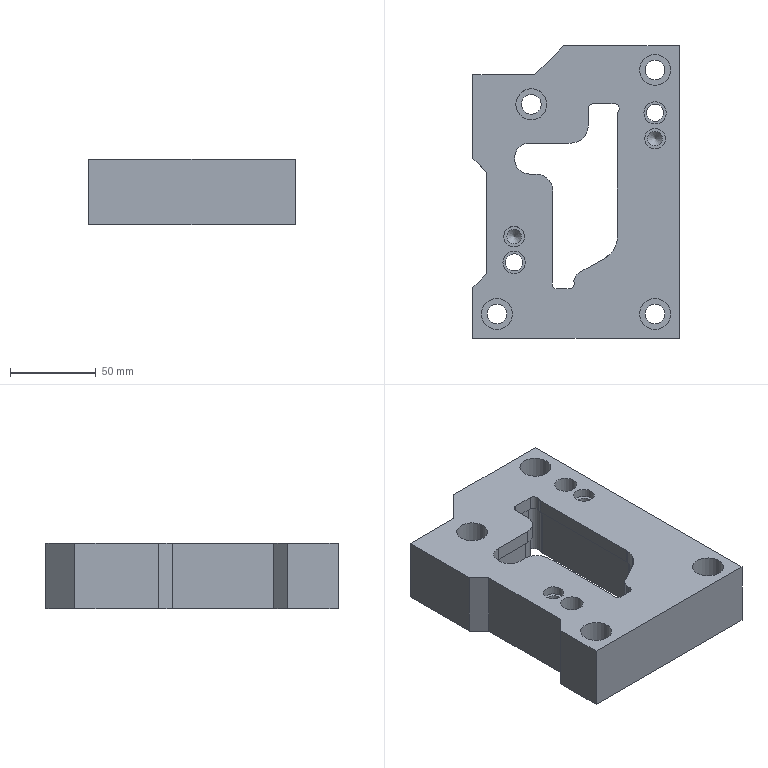Part | STEP file | lll_id274_x_t | 1 solid | 96 faces | box 120 x 170 x 38 mm | volume 536756 mm3 | cylinder 54 | plane 40 | cone 2 | commonest cylinder face diameters 6 x7 9 x4 11.509 x4 17.001 x4 18.008 x4 20.001 x4